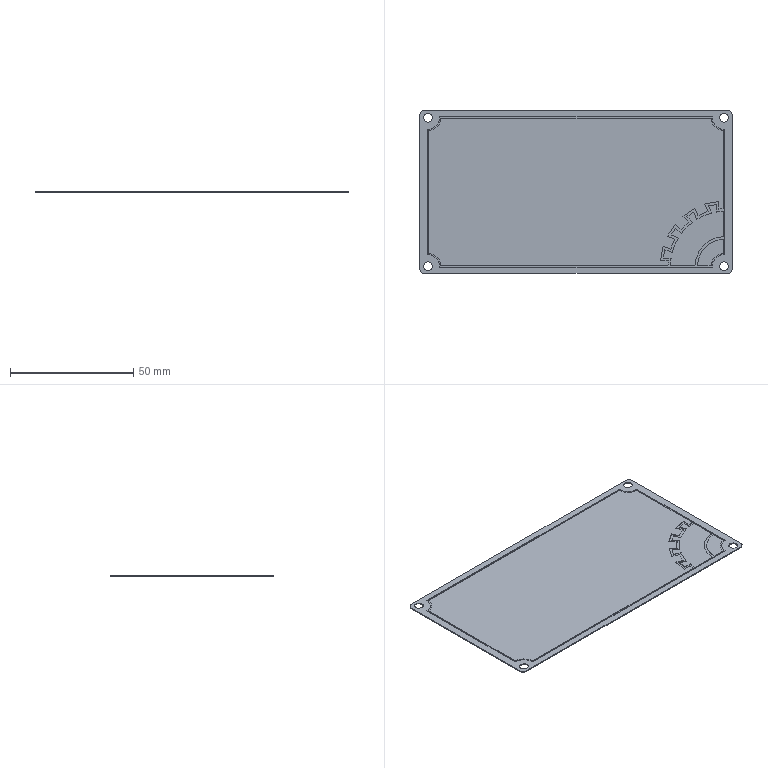Part | STEP file | 1 solid | 80 faces | box 126.7 x 66.1 x 0.4 mm | volume 3280 mm3 | plane 46 | cylinder 34 | commonest cylinder face diameters 3.6 x8 9.4 x6 4 x4 10.4 x4 22.436 x1 24.436 x1